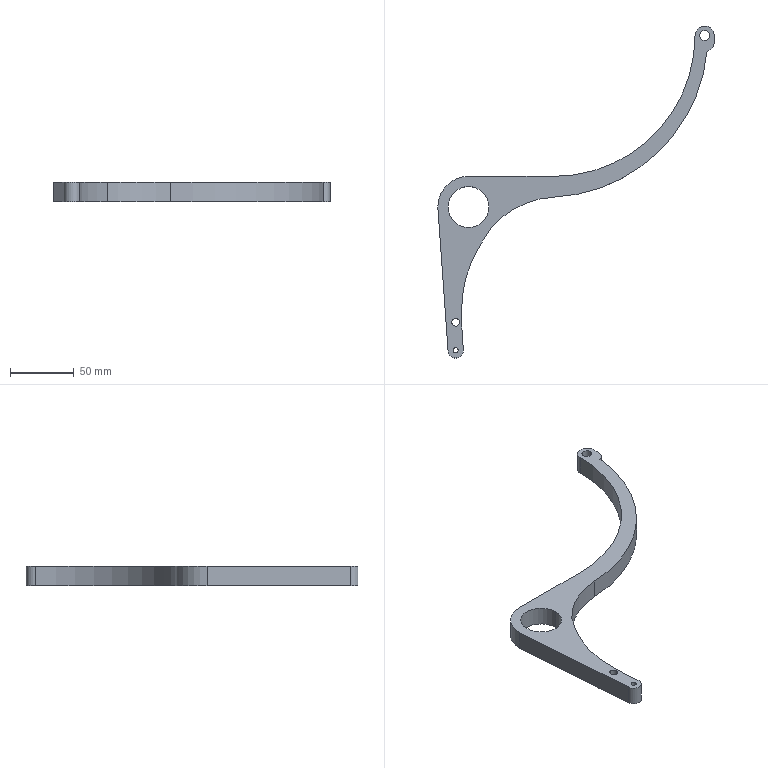Part | SolidWorks | features Extrusion 1 | 1 solid | 21 faces | box 216 x 259.5 x 15 mm | volume 91694 mm3 | cylinder 15 | plane 5 | spline 1 | commonest cylinder face diameters 4 x2 6 x2 7.838 x2 32 x2 12 x1 15 x1
STEP:
#1=CARTESIAN_POINT('',(-3.,22.,15.));
#2=VERTEX_POINT('',#1);
#3=CARTESIAN_POINT('',(3.,22.,15.));
#4=VERTEX_POINT('',#3);
#5=CARTESIAN_POINT('',(0.,22.,15.));
#6=DIRECTION('',(0.,0.,1.));
#7=DIRECTION('',(1.,0.,0.));
#8=AXIS2_PLACEMENT_3D('',#5,#6,#7);
#9=CIRCLE('',#8,3.);
#10=EDGE_CURVE('',#2,#4,#9,.T.);
#11=ORIENTED_EDGE('',*,*,#10,.T.);
#12=CARTESIAN_POINT('',(3.,22.,0.));
#13=VERTEX_POINT('',#12);
#14=CARTESIAN_POINT('',(3.,22.,15.));
#15=DIRECTION('',(0.,0.,-1.));
#16=VECTOR('',#15,1000.);
#17=LINE('',#14,#16);
#18=EDGE_CURVE('',#4,#13,#17,.T.);
#19=ORIENTED_EDGE('',*,*,#18,.T.);
#20=CARTESIAN_POINT('',(-3.,22.,0.));
#21=VERTEX_POINT('',#20);
#22=CARTESIAN_POINT('',(0.,22.,0.));
#23=DIRECTION('',(0.,0.,1.));
#24=DIRECTION('',(1.,0.,0.));
#25=AXIS2_PLACEMENT_3D('',#22,#23,#24);
#26=CIRCLE('',#25,3.);
#27=EDGE_CURVE('',#21,#13,#26,.T.);
#28=ORIENTED_EDGE('',*,*,#27,.F.);
#29=CARTESIAN_POINT('',(-3.,22.,15.));
#30=DIRECTION('',(0.,0.,-1.));
#31=VECTOR('',#30,1000.);
#32=LINE('',#29,#31);
#33=EDGE_CURVE('',#2,#21,#32,.T.);
#34=ORIENTED_EDGE('',*,*,#33,.F.);
#35=EDGE_LOOP('',(#11,#19,#28,#34));
#36=FACE_OUTER_BOUND('',#35,.T.);
#37=CARTESIAN_POINT('',(0.,22.,15.));
#38=DIRECTION('',(0.,0.,-1.));
#39=DIRECTION('',(-1.,0.,0.));
#40=AXIS2_PLACEMENT_3D('',#37,#38,#39);
#41=CYLINDRICAL_SURFACE('',#40,3.);
#42=ADVANCED_FACE('',(#36),#41,.F.);
#43=CARTESIAN_POINT('',(190.581,246.,15.));
#44=VERTEX_POINT('',#43);
#45=CARTESIAN_POINT('',(198.419,246.,15.));
#46=VERTEX_POINT('',#45);
#47=CARTESIAN_POINT('',(194.5,246.,15.));
#48=DIRECTION('',(0.,0.,1.));
#49=DIRECTION('',(1.,0.,0.));
#50=AXIS2_PLACEMENT_3D('',#47,#48,#49);
#51=CIRCLE('',#50,3.919);
#52=EDGE_CURVE('',#44,#46,#51,.T.);
#53=ORIENTED_EDGE('',*,*,#52,.T.);
#54=CARTESIAN_POINT('',(198.419,246.,0.));
#55=VERTEX_POINT('',#54);
#56=CARTESIAN_POINT('',(198.419,246.,15.));
#57=DIRECTION('',(0.,0.,-1.));
#58=VECTOR('',#57,1000.);
#59=LINE('',#56,#58);
#60=EDGE_CURVE('',#46,#55,#59,.T.);
#61=ORIENTED_EDGE('',*,*,#60,.T.);
#62=CARTESIAN_POINT('',(190.581,246.,0.));
#63=VERTEX_POINT('',#62);
#64=CARTESIAN_POINT('',(194.5,246.,0.));
#65=DIRECTION('',(0.,0.,1.));
#66=DIRECTION('',(1.,0.,0.));
#67=AXIS2_PLACEMENT_3D('',#64,#65,#66);
#68=CIRCLE('',#67,3.919);
#69=EDGE_CURVE('',#63,#55,#68,.T.);
#70=ORIENTED_EDGE('',*,*,#69,.F.);
#71=CARTESIAN_POINT('',(190.581,246.,15.));
#72=DIRECTION('',(0.,0.,-1.));
#73=VECTOR('',#72,1000.);
#74=LINE('',#71,#73);
#75=EDGE_CURVE('',#44,#63,#74,.T.);
#76=ORIENTED_EDGE('',*,*,#75,.F.);
#77=EDGE_LOOP('',(#53,#61,#70,#76));
#78=FACE_OUTER_BOUND('',#77,.T.);
#79=CARTESIAN_POINT('',(194.5,246.,15.));
#80=DIRECTION('',(0.,0.,-1.));
#81=DIRECTION('',(-1.,0.,0.));
#82=AXIS2_PLACEMENT_3D('',#79,#80,#81);
#83=CYLINDRICAL_SURFACE('',#82,3.919);
#84=ADVANCED_FACE('',(#78),#83,.F.);
#85=CARTESIAN_POINT('',(-6.,112.,15.));
#86=VERTEX_POINT('',#85);
#87=CARTESIAN_POINT('',(26.,112.,15.));
#88=VERTEX_POINT('',#87);
#89=CARTESIAN_POINT('',(10.,112.,15.));
#90=DIRECTION('',(0.,0.,1.));
#91=DIRECTION('',(1.,0.,0.));
#92=AXIS2_PLACEMENT_3D('',#89,#90,#91);
#93=CIRCLE('',#92,16.);
#94=EDGE_CURVE('',#86,#88,#93,.T.);
#95=ORIENTED_EDGE('',*,*,#94,.T.);
#96=CARTESIAN_POINT('',(26.,112.,0.));
#97=VERTEX_POINT('',#96);
#98=CARTESIAN_POINT('',(26.,112.,15.));
#99=DIRECTION('',(0.,0.,-1.));
#100=VECTOR('',#99,1000.);
#101=LINE('',#98,#100);
#102=EDGE_CURVE('',#88,#97,#101,.T.);
#103=ORIENTED_EDGE('',*,*,#102,.T.);
#104=CARTESIAN_POINT('',(-6.,112.,0.));
#105=VERTEX_POINT('',#104);
#106=CARTESIAN_POINT('',(10.,112.,0.));
#107=DIRECTION('',(0.,0.,1.));
#108=DIRECTION('',(1.,0.,0.));
#109=AXIS2_PLACEMENT_3D('',#106,#107,#108);
#110=CIRCLE('',#109,16.);
#111=EDGE_CURVE('',#105,#97,#110,.T.);
#112=ORIENTED_EDGE('',*,*,#111,.F.);
#113=CARTESIAN_POINT('',(-6.,112.,15.));
#114=DIRECTION('',(0.,0.,-1.));
#115=VECTOR('',#114,1000.);
#116=LINE('',#113,#115);
#117=EDGE_CURVE('',#86,#105,#116,.T.);
#118=ORIENTED_EDGE('',*,*,#117,.F.);
#119=EDGE_LOOP('',(#95,#103,#112,#118));
#120=FACE_OUTER_BOUND('',#119,.T.);
#121=CARTESIAN_POINT('',(10.,112.,15.));
#122=DIRECTION('',(0.,0.,-1.));
#123=DIRECTION('',(-1.,0.,0.));
#124=AXIS2_PLACEMENT_3D('',#121,#122,#123);
#125=CYLINDRICAL_SURFACE('',#124,16.);
#126=ADVANCED_FACE('',(#120),#125,.F.);
#127=CARTESIAN_POINT('',(-2.,0.,15.));
#128=VERTEX_POINT('',#127);
#129=CARTESIAN_POINT('',(2.,0.,15.));
#130=VERTEX_POINT('',#129);
#131=CARTESIAN_POINT('',(0.,0.,15.));
#132=DIRECTION('',(0.,0.,1.));
#133=DIRECTION('',(1.,0.,0.));
#134=AXIS2_PLACEMENT_3D('',#131,#132,#133);
#135=CIRCLE('',#134,2.);
#136=EDGE_CURVE('',#128,#130,#135,.T.);
#137=ORIENTED_EDGE('',*,*,#136,.T.);
#138=CARTESIAN_POINT('',(2.,0.,0.));
#139=VERTEX_POINT('',#138);
#140=CARTESIAN_POINT('',(2.,0.,15.));
#141=DIRECTION('',(0.,0.,-1.));
#142=VECTOR('',#141,1000.);
#143=LINE('',#140,#142);
#144=EDGE_CURVE('',#130,#139,#143,.T.);
#145=ORIENTED_EDGE('',*,*,#144,.T.);
#146=CARTESIAN_POINT('',(-2.,0.,0.));
#147=VERTEX_POINT('',#146);
#148=CARTESIAN_POINT('',(0.,0.,0.));
#149=DIRECTION('',(0.,0.,1.));
#150=DIRECTION('',(1.,0.,0.));
#151=AXIS2_PLACEMENT_3D('',#148,#149,#150);
#152=CIRCLE('',#151,2.);
#153=EDGE_CURVE('',#147,#139,#152,.T.);
#154=ORIENTED_EDGE('',*,*,#153,.F.);
#155=CARTESIAN_POINT('',(-2.,0.,15.));
#156=DIRECTION('',(0.,0.,-1.));
#157=VECTOR('',#156,1000.);
#158=LINE('',#155,#157);
#159=EDGE_CURVE('',#128,#147,#158,.T.);
#160=ORIENTED_EDGE('',*,*,#159,.F.);
#161=EDGE_LOOP('',(#137,#145,#154,#160));
#162=FACE_OUTER_BOUND('',#161,.T.);
#163=CARTESIAN_POINT('',(0.,0.,15.));
#164=DIRECTION('',(0.,0.,-1.));
#165=DIRECTION('',(-1.,0.,0.));
#166=AXIS2_PLACEMENT_3D('',#163,#164,#165);
#167=CYLINDRICAL_SURFACE('',#166,2.);
#168=ADVANCED_FACE('',(#162),#167,.F.);
#169=ORIENTED_EDGE('',*,*,#52,.F.);
#170=CARTESIAN_POINT('',(194.5,246.,15.));
#171=DIRECTION('',(0.,0.,1.));
#172=DIRECTION('',(1.,0.,0.));
#173=AXIS2_PLACEMENT_3D('',#170,#171,#172);
#174=CIRCLE('',#173,3.919);
#175=EDGE_CURVE('',#46,#44,#174,.T.);
#176=ORIENTED_EDGE('',*,*,#175,.F.);
#177=EDGE_LOOP('',(#169,#176));
#178=FACE_BOUND('',#177,.T.);
#179=ORIENTED_EDGE('',*,*,#136,.F.);
#180=CARTESIAN_POINT('',(0.,0.,15.));
#181=DIRECTION('',(0.,0.,1.));
#182=DIRECTION('',(1.,0.,0.));
#183=AXIS2_PLACEMENT_3D('',#180,#181,#182);
#184=CIRCLE('',#183,2.);
#185=EDGE_CURVE('',#130,#128,#184,.T.);
#186=ORIENTED_EDGE('',*,*,#185,.F.);
#187=EDGE_LOOP('',(#179,#186));
#188=FACE_BOUND('',#187,.T.);
#189=CARTESIAN_POINT('',(10.,136.,15.));
#190=VERTEX_POINT('',#189);
#191=CARTESIAN_POINT('',(-14.,112.,15.));
#192=VERTEX_POINT('',#191);
#193=CARTESIAN_POINT('',(10.,112.,15.));
#194=DIRECTION('',(0.,0.,1.));
#195=DIRECTION('',(1.,0.,0.));
#196=AXIS2_PLACEMENT_3D('',#193,#194,#195);
#197=CIRCLE('',#196,24.);
#198=EDGE_CURVE('',#190,#192,#197,.T.);
#199=ORIENTED_EDGE('',*,*,#198,.T.);
#200=CARTESIAN_POINT('',(-6.,0.,15.));
#201=VERTEX_POINT('',#200);
#202=CARTESIAN_POINT('',(-14.,112.,15.));
#203=DIRECTION('',(0.07125,-0.9975,0.));
#204=VECTOR('',#203,1000.);
#205=LINE('',#202,#204);
#206=EDGE_CURVE('',#192,#201,#205,.T.);
#207=ORIENTED_EDGE('',*,*,#206,.T.);
#208=CARTESIAN_POINT('',(6.,0.,15.));
#209=VERTEX_POINT('',#208);
#210=CARTESIAN_POINT('',(0.,0.,15.));
#211=DIRECTION('',(0.,0.,1.));
#212=DIRECTION('',(1.,0.,0.));
#213=AXIS2_PLACEMENT_3D('',#210,#211,#212);
#214=CIRCLE('',#213,6.);
#215=EDGE_CURVE('',#201,#209,#214,.T.);
#216=ORIENTED_EDGE('',*,*,#215,.T.);
#217=CARTESIAN_POINT('',(28.005,96.131,15.));
#218=VERTEX_POINT('',#217);
#219=CARTESIAN_POINT('',(6.,0.,15.));
#220=CARTESIAN_POINT('',(1.589,45.681,15.));
#221=CARTESIAN_POINT('',(5.604,63.643,15.));
#222=CARTESIAN_POINT('',(28.005,96.131,15.));
#223=B_SPLINE_CURVE_WITH_KNOTS('',3,(#219,#220,#221,#222),.UNSPECIFIED.,.F.,.F.,(4,4),(0.,0.7882),.UNSPECIFIED.);
#224=EDGE_CURVE('',#209,#218,#223,.T.);
#225=ORIENTED_EDGE('',*,*,#224,.T.);
#226=CARTESIAN_POINT('',(77.,119.767,15.));
#227=VERTEX_POINT('',#226);
#228=CARTESIAN_POINT('',(80.543,49.825,15.));
#229=DIRECTION('',(0.,0.,-1.));
#230=DIRECTION('',(1.,0.,0.));
#231=AXIS2_PLACEMENT_3D('',#228,#229,#230);
#232=CIRCLE('',#231,70.032);
#233=EDGE_CURVE('',#218,#227,#232,.T.);
#234=ORIENTED_EDGE('',*,*,#233,.T.);
#235=CARTESIAN_POINT('',(196.38,233.495,15.));
#236=VERTEX_POINT('',#235);
#237=CARTESIAN_POINT('',(70.606,246.,15.));
#238=DIRECTION('',(0.,0.,1.));
#239=DIRECTION('',(1.,0.,0.));
#240=AXIS2_PLACEMENT_3D('',#237,#238,#239);
#241=CIRCLE('',#240,126.394);
#242=EDGE_CURVE('',#227,#236,#241,.T.);
#243=ORIENTED_EDGE('',*,*,#242,.T.);
#244=CARTESIAN_POINT('',(202.,241.,15.));
#245=VERTEX_POINT('',#244);
#246=CARTESIAN_POINT('',(194.179,241.,15.));
#247=DIRECTION('',(0.,0.,1.));
#248=DIRECTION('',(1.,0.,0.));
#249=AXIS2_PLACEMENT_3D('',#246,#247,#248);
#250=CIRCLE('',#249,7.821);
#251=EDGE_CURVE('',#236,#245,#250,.T.);
#252=ORIENTED_EDGE('',*,*,#251,.T.);
#253=CARTESIAN_POINT('',(202.,246.,15.));
#254=VERTEX_POINT('',#253);
#255=CARTESIAN_POINT('',(202.,246.,15.));
#256=DIRECTION('',(0.,1.,0.));
#257=VECTOR('',#256,1000.);
#258=LINE('',#255,#257);
#259=EDGE_CURVE('',#245,#254,#258,.T.);
#260=ORIENTED_EDGE('',*,*,#259,.T.);
#261=CARTESIAN_POINT('',(187.,246.,15.));
#262=VERTEX_POINT('',#261);
#263=CARTESIAN_POINT('',(194.5,246.,15.));
#264=DIRECTION('',(0.,0.,1.));
#265=DIRECTION('',(1.,0.,0.));
#266=AXIS2_PLACEMENT_3D('',#263,#264,#265);
#267=CIRCLE('',#266,7.5);
#268=EDGE_CURVE('',#254,#262,#267,.T.);
#269=ORIENTED_EDGE('',*,*,#268,.T.);
#270=CARTESIAN_POINT('',(77.,136.,15.));
#271=VERTEX_POINT('',#270);
#272=CARTESIAN_POINT('',(77.,246.,15.));
#273=DIRECTION('',(0.,0.,-1.));
#274=DIRECTION('',(1.,0.,0.));
#275=AXIS2_PLACEMENT_3D('',#272,#273,#274);
#276=CIRCLE('',#275,110.);
#277=EDGE_CURVE('',#262,#271,#276,.T.);
#278=ORIENTED_EDGE('',*,*,#277,.T.);
#279=CARTESIAN_POINT('',(10.,136.,15.));
#280=DIRECTION('',(-1.,0.,0.));
#281=VECTOR('',#280,1000.);
#282=LINE('',#279,#281);
#283=EDGE_CURVE('',#271,#190,#282,.T.);
#284=ORIENTED_EDGE('',*,*,#283,.T.);
#285=EDGE_LOOP('',(#199,#207,#216,#225,#234,#243,#252,#260,#269,#278,#284));
#286=FACE_OUTER_BOUND('',#285,.T.);
#287=ORIENTED_EDGE('',*,*,#94,.F.);
#288=CARTESIAN_POINT('',(10.,112.,15.));
#289=DIRECTION('',(0.,0.,1.));
#290=DIRECTION('',(1.,0.,0.));
#291=AXIS2_PLACEMENT_3D('',#288,#289,#290);
#292=CIRCLE('',#291,16.);
#293=EDGE_CURVE('',#88,#86,#292,.T.);
#294=ORIENTED_EDGE('',*,*,#293,.F.);
#295=EDGE_LOOP('',(#287,#294));
#296=FACE_BOUND('',#295,.T.);
#297=ORIENTED_EDGE('',*,*,#10,.F.);
#298=CARTESIAN_POINT('',(0.,22.,15.));
#299=DIRECTION('',(0.,0.,1.));
#300=DIRECTION('',(1.,0.,0.));
#301=AXIS2_PLACEMENT_3D('',#298,#299,#300);
#302=CIRCLE('',#301,3.);
#303=EDGE_CURVE('',#4,#2,#302,.T.);
#304=ORIENTED_EDGE('',*,*,#303,.F.);
#305=EDGE_LOOP('',(#297,#304));
#306=FACE_BOUND('',#305,.T.);
#307=CARTESIAN_POINT('',(10.,112.,15.));
#308=DIRECTION('',(0.,0.,1.));
#309=DIRECTION('',(1.,0.,0.));
#310=AXIS2_PLACEMENT_3D('',#307,#308,#309);
#311=PLANE('',#310);
#312=ADVANCED_FACE('',(#178,#188,#286,#296,#306),#311,.T.);
#313=CARTESIAN_POINT('',(10.,136.,0.));
#314=VERTEX_POINT('',#313);
#315=CARTESIAN_POINT('',(-14.,112.,0.));
#316=VERTEX_POINT('',#315);
#317=CARTESIAN_POINT('',(10.,112.,0.));
#318=DIRECTION('',(0.,0.,1.));
#319=DIRECTION('',(1.,0.,0.));
#320=AXIS2_PLACEMENT_3D('',#317,#318,#319);
#321=CIRCLE('',#320,24.);
#322=EDGE_CURVE('',#314,#316,#321,.T.);
#323=ORIENTED_EDGE('',*,*,#322,.F.);
#324=CARTESIAN_POINT('',(77.,136.,0.));
#325=VERTEX_POINT('',#324);
#326=CARTESIAN_POINT('',(10.,136.,0.));
#327=DIRECTION('',(-1.,0.,0.));
#328=VECTOR('',#327,1000.);
#329=LINE('',#326,#328);
#330=EDGE_CURVE('',#325,#314,#329,.T.);
#331=ORIENTED_EDGE('',*,*,#330,.F.);
#332=CARTESIAN_POINT('',(187.,246.,0.));
#333=VERTEX_POINT('',#332);
#334=CARTESIAN_POINT('',(77.,246.,0.));
#335=DIRECTION('',(0.,0.,-1.));
#336=DIRECTION('',(1.,0.,0.));
#337=AXIS2_PLACEMENT_3D('',#334,#335,#336);
#338=CIRCLE('',#337,110.);
#339=EDGE_CURVE('',#333,#325,#338,.T.);
#340=ORIENTED_EDGE('',*,*,#339,.F.);
#341=CARTESIAN_POINT('',(202.,246.,0.));
#342=VERTEX_POINT('',#341);
#343=CARTESIAN_POINT('',(194.5,246.,0.));
#344=DIRECTION('',(0.,0.,1.));
#345=DIRECTION('',(1.,0.,0.));
#346=AXIS2_PLACEMENT_3D('',#343,#344,#345);
#347=CIRCLE('',#346,7.5);
#348=EDGE_CURVE('',#342,#333,#347,.T.);
#349=ORIENTED_EDGE('',*,*,#348,.F.);
#350=CARTESIAN_POINT('',(202.,241.,0.));
#351=VERTEX_POINT('',#350);
#352=CARTESIAN_POINT('',(202.,246.,0.));
#353=DIRECTION('',(0.,1.,0.));
#354=VECTOR('',#353,1000.);
#355=LINE('',#352,#354);
#356=EDGE_CURVE('',#351,#342,#355,.T.);
#357=ORIENTED_EDGE('',*,*,#356,.F.);
#358=CARTESIAN_POINT('',(196.38,233.495,0.));
#359=VERTEX_POINT('',#358);
#360=CARTESIAN_POINT('',(194.179,241.,0.));
#361=DIRECTION('',(0.,0.,1.));
#362=DIRECTION('',(1.,0.,0.));
#363=AXIS2_PLACEMENT_3D('',#360,#361,#362);
#364=CIRCLE('',#363,7.821);
#365=EDGE_CURVE('',#359,#351,#364,.T.);
#366=ORIENTED_EDGE('',*,*,#365,.F.);
#367=CARTESIAN_POINT('',(77.,119.767,0.));
#368=VERTEX_POINT('',#367);
#369=CARTESIAN_POINT('',(70.606,246.,0.));
#370=DIRECTION('',(0.,0.,1.));
#371=DIRECTION('',(1.,0.,0.));
#372=AXIS2_PLACEMENT_3D('',#369,#370,#371);
#373=CIRCLE('',#372,126.394);
#374=EDGE_CURVE('',#368,#359,#373,.T.);
#375=ORIENTED_EDGE('',*,*,#374,.F.);
#376=CARTESIAN_POINT('',(28.005,96.131,0.));
#377=VERTEX_POINT('',#376);
#378=CARTESIAN_POINT('',(80.543,49.825,0.));
#379=DIRECTION('',(0.,0.,-1.));
#380=DIRECTION('',(1.,0.,0.));
#381=AXIS2_PLACEMENT_3D('',#378,#379,#380);
#382=CIRCLE('',#381,70.032);
#383=EDGE_CURVE('',#377,#368,#382,.T.);
#384=ORIENTED_EDGE('',*,*,#383,.F.);
#385=CARTESIAN_POINT('',(6.,0.,0.));
#386=VERTEX_POINT('',#385);
#387=CARTESIAN_POINT('',(6.,0.,0.));
#388=CARTESIAN_POINT('',(1.589,45.681,0.));
#389=CARTESIAN_POINT('',(5.604,63.643,0.));
#390=CARTESIAN_POINT('',(28.005,96.131,0.));
#391=B_SPLINE_CURVE_WITH_KNOTS('',3,(#387,#388,#389,#390),.UNSPECIFIED.,.F.,.F.,(4,4),(0.,0.7882),.UNSPECIFIED.);
#392=EDGE_CURVE('',#386,#377,#391,.T.);
#393=ORIENTED_EDGE('',*,*,#392,.F.);
#394=CARTESIAN_POINT('',(-6.,0.,0.));
#395=VERTEX_POINT('',#394);
#396=CARTESIAN_POINT('',(0.,0.,0.));
#397=DIRECTION('',(0.,0.,1.));
#398=DIRECTION('',(1.,0.,0.));
#399=AXIS2_PLACEMENT_3D('',#396,#397,#398);
#400=CIRCLE('',#399,6.);
#401=EDGE_CURVE('',#395,#386,#400,.T.);
#402=ORIENTED_EDGE('',*,*,#401,.F.);
#403=CARTESIAN_POINT('',(-14.,112.,0.));
#404=DIRECTION('',(0.07125,-0.9975,0.));
#405=VECTOR('',#404,1000.);
#406=LINE('',#403,#405);
#407=EDGE_CURVE('',#316,#395,#406,.T.);
#408=ORIENTED_EDGE('',*,*,#407,.F.);
#409=EDGE_LOOP('',(#323,#331,#340,#349,#357,#366,#375,#384,#393,#402,#408));
#410=FACE_OUTER_BOUND('',#409,.T.);
#411=ORIENTED_EDGE('',*,*,#153,.T.);
#412=CARTESIAN_POINT('',(0.,0.,0.));
#413=DIRECTION('',(0.,0.,1.));
#414=DIRECTION('',(1.,0.,0.));
#415=AXIS2_PLACEMENT_3D('',#412,#413,#414);
#416=CIRCLE('',#415,2.);
#417=EDGE_CURVE('',#139,#147,#416,.T.);
#418=ORIENTED_EDGE('',*,*,#417,.T.);
#419=EDGE_LOOP('',(#411,#418));
#420=FACE_BOUND('',#419,.T.);
#421=ORIENTED_EDGE('',*,*,#111,.T.);
#422=CARTESIAN_POINT('',(10.,112.,0.));
#423=DIRECTION('',(0.,0.,1.));
#424=DIRECTION('',(1.,0.,0.));
#425=AXIS2_PLACEMENT_3D('',#422,#423,#424);
#426=CIRCLE('',#425,16.);
#427=EDGE_CURVE('',#97,#105,#426,.T.);
#428=ORIENTED_EDGE('',*,*,#427,.T.);
#429=EDGE_LOOP('',(#421,#428));
#430=FACE_BOUND('',#429,.T.);
#431=ORIENTED_EDGE('',*,*,#69,.T.);
#432=CARTESIAN_POINT('',(194.5,246.,0.));
#433=DIRECTION('',(0.,0.,1.));
#434=DIRECTION('',(1.,0.,0.));
#435=AXIS2_PLACEMENT_3D('',#432,#433,#434);
#436=CIRCLE('',#435,3.919);
#437=EDGE_CURVE('',#55,#63,#436,.T.);
#438=ORIENTED_EDGE('',*,*,#437,.T.);
#439=EDGE_LOOP('',(#431,#438));
#440=FACE_BOUND('',#439,.T.);
#441=ORIENTED_EDGE('',*,*,#27,.T.);
#442=CARTESIAN_POINT('',(0.,22.,0.));
#443=DIRECTION('',(0.,0.,1.));
#444=DIRECTION('',(1.,0.,0.));
#445=AXIS2_PLACEMENT_3D('',#442,#443,#444);
#446=CIRCLE('',#445,3.);
#447=EDGE_CURVE('',#13,#21,#446,.T.);
#448=ORIENTED_EDGE('',*,*,#447,.T.);
#449=EDGE_LOOP('',(#441,#448));
#450=FACE_BOUND('',#449,.T.);
#451=CARTESIAN_POINT('',(10.,112.,0.));
#452=DIRECTION('',(0.,0.,1.));
#453=DIRECTION('',(1.,0.,0.));
#454=AXIS2_PLACEMENT_3D('',#451,#452,#453);
#455=PLANE('',#454);
#456=ADVANCED_FACE('',(#410,#420,#430,#440,#450),#455,.F.);
#457=ORIENTED_EDGE('',*,*,#322,.T.);
#458=CARTESIAN_POINT('',(-14.,112.,15.));
#459=DIRECTION('',(0.,0.,-1.));
#460=VECTOR('',#459,1000.);
#461=LINE('',#458,#460);
#462=EDGE_CURVE('',#192,#316,#461,.T.);
#463=ORIENTED_EDGE('',*,*,#462,.F.);
#464=ORIENTED_EDGE('',*,*,#198,.F.);
#465=CARTESIAN_POINT('',(10.,136.,15.));
#466=DIRECTION('',(0.,0.,-1.));
#467=VECTOR('',#466,1000.);
#468=LINE('',#465,#467);
#469=EDGE_CURVE('',#190,#314,#468,.T.);
#470=ORIENTED_EDGE('',*,*,#469,.T.);
#471=EDGE_LOOP('',(#457,#463,#464,#470));
#472=FACE_OUTER_BOUND('',#471,.T.);
#473=CARTESIAN_POINT('',(10.,112.,15.));
#474=DIRECTION('',(0.,0.,-1.));
#475=DIRECTION('',(-1.,0.,0.));
#476=AXIS2_PLACEMENT_3D('',#473,#474,#475);
#477=CYLINDRICAL_SURFACE('',#476,24.);
#478=ADVANCED_FACE('',(#472),#477,.T.);
#479=ORIENTED_EDGE('',*,*,#407,.T.);
#480=CARTESIAN_POINT('',(-6.,0.,15.));
#481=DIRECTION('',(0.,0.,-1.));
#482=VECTOR('',#481,1000.);
#483=LINE('',#480,#482);
#484=EDGE_CURVE('',#201,#395,#483,.T.);
#485=ORIENTED_EDGE('',*,*,#484,.F.);
#486=ORIENTED_EDGE('',*,*,#206,.F.);
#487=ORIENTED_EDGE('',*,*,#462,.T.);
#488=EDGE_LOOP('',(#479,#485,#486,#487));
#489=FACE_OUTER_BOUND('',#488,.T.);
#490=CARTESIAN_POINT('',(-14.,112.,15.));
#491=DIRECTION('',(0.9975,0.07125,0.));
#492=DIRECTION('',(-0.07125,0.9975,0.));
#493=AXIS2_PLACEMENT_3D('',#490,#491,#492);
#494=PLANE('',#493);
#495=ADVANCED_FACE('',(#489),#494,.F.);
#496=ORIENTED_EDGE('',*,*,#401,.T.);
#497=CARTESIAN_POINT('',(6.,0.,15.));
#498=DIRECTION('',(0.,0.,-1.));
#499=VECTOR('',#498,1000.);
#500=LINE('',#497,#499);
#501=EDGE_CURVE('',#209,#386,#500,.T.);
#502=ORIENTED_EDGE('',*,*,#501,.F.);
#503=ORIENTED_EDGE('',*,*,#215,.F.);
#504=ORIENTED_EDGE('',*,*,#484,.T.);
#505=EDGE_LOOP('',(#496,#502,#503,#504));
#506=FACE_OUTER_BOUND('',#505,.T.);
#507=CARTESIAN_POINT('',(0.,0.,15.));
#508=DIRECTION('',(0.,0.,-1.));
#509=DIRECTION('',(-1.,0.,0.));
#510=AXIS2_PLACEMENT_3D('',#507,#508,#509);
#511=CYLINDRICAL_SURFACE('',#510,6.);
#512=ADVANCED_FACE('',(#506),#511,.T.);
#513=ORIENTED_EDGE('',*,*,#392,.T.);
#514=CARTESIAN_POINT('',(28.005,96.131,15.));
#515=DIRECTION('',(0.,0.,-1.));
#516=VECTOR('',#515,1000.);
#517=LINE('',#514,#516);
#518=EDGE_CURVE('',#218,#377,#517,.T.);
#519=ORIENTED_EDGE('',*,*,#518,.F.);
#520=ORIENTED_EDGE('',*,*,#224,.F.);
#521=ORIENTED_EDGE('',*,*,#501,.T.);
#522=EDGE_LOOP('',(#513,#519,#520,#521));
#523=FACE_OUTER_BOUND('',#522,.T.);
#524=CARTESIAN_POINT('',(6.,0.,15.));
#525=CARTESIAN_POINT('',(6.,0.,0.));
#526=CARTESIAN_POINT('',(1.589,45.681,15.));
#527=CARTESIAN_POINT('',(1.589,45.681,0.));
#528=CARTESIAN_POINT('',(5.604,63.643,15.));
#529=CARTESIAN_POINT('',(5.604,63.643,0.));
#530=CARTESIAN_POINT('',(28.005,96.131,15.));
#531=CARTESIAN_POINT('',(28.005,96.131,0.));
#532=B_SPLINE_SURFACE_WITH_KNOTS('',3,1,((#524,#525),(#526,#527),(#528,#529),(#530,#531)),.UNSPECIFIED.,.F.,.F.,.F.,(4,4),(2,2),(0.,0.7882),(0.,1.),.UNSPECIFIED.);
#533=ADVANCED_FACE('',(#523),#532,.F.);
#534=ORIENTED_EDGE('',*,*,#383,.T.);
#535=CARTESIAN_POINT('',(77.,119.767,15.));
#536=DIRECTION('',(0.,0.,-1.));
#537=VECTOR('',#536,1000.);
#538=LINE('',#535,#537);
#539=EDGE_CURVE('',#227,#368,#538,.T.);
#540=ORIENTED_EDGE('',*,*,#539,.F.);
#541=ORIENTED_EDGE('',*,*,#233,.F.);
#542=ORIENTED_EDGE('',*,*,#518,.T.);
#543=EDGE_LOOP('',(#534,#540,#541,#542));
#544=FACE_OUTER_BOUND('',#543,.T.);
#545=CARTESIAN_POINT('',(80.543,49.825,15.));
#546=DIRECTION('',(0.,0.,-1.));
#547=DIRECTION('',(-1.,0.,0.));
#548=AXIS2_PLACEMENT_3D('',#545,#546,#547);
#549=CYLINDRICAL_SURFACE('',#548,70.032);
#550=ADVANCED_FACE('',(#544),#549,.F.);
#551=ORIENTED_EDGE('',*,*,#374,.T.);
#552=CARTESIAN_POINT('',(196.38,233.495,15.));
#553=DIRECTION('',(0.,0.,-1.));
#554=VECTOR('',#553,1000.);
#555=LINE('',#552,#554);
#556=EDGE_CURVE('',#236,#359,#555,.T.);
#557=ORIENTED_EDGE('',*,*,#556,.F.);
#558=ORIENTED_EDGE('',*,*,#242,.F.);
#559=ORIENTED_EDGE('',*,*,#539,.T.);
#560=EDGE_LOOP('',(#551,#557,#558,#559));
#561=FACE_OUTER_BOUND('',#560,.T.);
#562=CARTESIAN_POINT('',(70.606,246.,15.));
#563=DIRECTION('',(0.,0.,-1.));
#564=DIRECTION('',(-1.,0.,0.));
#565=AXIS2_PLACEMENT_3D('',#562,#563,#564);
#566=CYLINDRICAL_SURFACE('',#565,126.394);
#567=ADVANCED_FACE('',(#561),#566,.T.);
#568=ORIENTED_EDGE('',*,*,#365,.T.);
#569=CARTESIAN_POINT('',(202.,241.,15.));
#570=DIRECTION('',(0.,0.,-1.));
#571=VECTOR('',#570,1000.);
#572=LINE('',#569,#571);
#573=EDGE_CURVE('',#245,#351,#572,.T.);
#574=ORIENTED_EDGE('',*,*,#573,.F.);
#575=ORIENTED_EDGE('',*,*,#251,.F.);
#576=ORIENTED_EDGE('',*,*,#556,.T.);
#577=EDGE_LOOP('',(#568,#574,#575,#576));
#578=FACE_OUTER_BOUND('',#577,.T.);
#579=CARTESIAN_POINT('',(194.179,241.,15.));
#580=DIRECTION('',(0.,0.,-1.));
#581=DIRECTION('',(-1.,0.,0.));
#582=AXIS2_PLACEMENT_3D('',#579,#580,#581);
#583=CYLINDRICAL_SURFACE('',#582,7.821);
#584=ADVANCED_FACE('',(#578),#583,.T.);
#585=ORIENTED_EDGE('',*,*,#356,.T.);
#586=CARTESIAN_POINT('',(202.,246.,15.));
#587=DIRECTION('',(0.,0.,-1.));
#588=VECTOR('',#587,1000.);
#589=LINE('',#586,#588);
#590=EDGE_CURVE('',#254,#342,#589,.T.);
#591=ORIENTED_EDGE('',*,*,#590,.F.);
#592=ORIENTED_EDGE('',*,*,#259,.F.);
#593=ORIENTED_EDGE('',*,*,#573,.T.);
#594=EDGE_LOOP('',(#585,#591,#592,#593));
#595=FACE_OUTER_BOUND('',#594,.T.);
#596=CARTESIAN_POINT('',(202.,246.,15.));
#597=DIRECTION('',(-1.,0.,0.));
#598=DIRECTION('',(0.,0.,1.));
#599=AXIS2_PLACEMENT_3D('',#596,#597,#598);
#600=PLANE('',#599);
#601=ADVANCED_FACE('',(#595),#600,.F.);
#602=ORIENTED_EDGE('',*,*,#348,.T.);
#603=CARTESIAN_POINT('',(187.,246.,15.));
#604=DIRECTION('',(0.,0.,-1.));
#605=VECTOR('',#604,1000.);
#606=LINE('',#603,#605);
#607=EDGE_CURVE('',#262,#333,#606,.T.);
#608=ORIENTED_EDGE('',*,*,#607,.F.);
#609=ORIENTED_EDGE('',*,*,#268,.F.);
#610=ORIENTED_EDGE('',*,*,#590,.T.);
#611=EDGE_LOOP('',(#602,#608,#609,#610));
#612=FACE_OUTER_BOUND('',#611,.T.);
#613=CARTESIAN_POINT('',(194.5,246.,15.));
#614=DIRECTION('',(0.,0.,-1.));
#615=DIRECTION('',(-1.,0.,0.));
#616=AXIS2_PLACEMENT_3D('',#613,#614,#615);
#617=CYLINDRICAL_SURFACE('',#616,7.5);
#618=ADVANCED_FACE('',(#612),#617,.T.);
#619=ORIENTED_EDGE('',*,*,#339,.T.);
#620=CARTESIAN_POINT('',(77.,136.,15.));
#621=DIRECTION('',(0.,0.,-1.));
#622=VECTOR('',#621,1000.);
#623=LINE('',#620,#622);
#624=EDGE_CURVE('',#271,#325,#623,.T.);
#625=ORIENTED_EDGE('',*,*,#624,.F.);
#626=ORIENTED_EDGE('',*,*,#277,.F.);
#627=ORIENTED_EDGE('',*,*,#607,.T.);
#628=EDGE_LOOP('',(#619,#625,#626,#627));
#629=FACE_OUTER_BOUND('',#628,.T.);
#630=CARTESIAN_POINT('',(77.,246.,15.));
#631=DIRECTION('',(0.,0.,-1.));
#632=DIRECTION('',(-1.,0.,0.));
#633=AXIS2_PLACEMENT_3D('',#630,#631,#632);
#634=CYLINDRICAL_SURFACE('',#633,110.);
#635=ADVANCED_FACE('',(#629),#634,.F.);
#636=ORIENTED_EDGE('',*,*,#330,.T.);
#637=ORIENTED_EDGE('',*,*,#469,.F.);
#638=ORIENTED_EDGE('',*,*,#283,.F.);
#639=ORIENTED_EDGE('',*,*,#624,.T.);
#640=EDGE_LOOP('',(#636,#637,#638,#639));
#641=FACE_OUTER_BOUND('',#640,.T.);
#642=CARTESIAN_POINT('',(10.,136.,15.));
#643=DIRECTION('',(0.,-1.,0.));
#644=DIRECTION('',(0.,0.,-1.));
#645=AXIS2_PLACEMENT_3D('',#642,#643,#644);
#646=PLANE('',#645);
#647=ADVANCED_FACE('',(#641),#646,.F.);
#648=ORIENTED_EDGE('',*,*,#144,.F.);
#649=ORIENTED_EDGE('',*,*,#185,.T.);
#650=ORIENTED_EDGE('',*,*,#159,.T.);
#651=ORIENTED_EDGE('',*,*,#417,.F.);
#652=EDGE_LOOP('',(#648,#649,#650,#651));
#653=FACE_OUTER_BOUND('',#652,.T.);
#654=CARTESIAN_POINT('',(0.,0.,15.));
#655=DIRECTION('',(0.,0.,-1.));
#656=DIRECTION('',(-1.,0.,0.));
#657=AXIS2_PLACEMENT_3D('',#654,#655,#656);
#658=CYLINDRICAL_SURFACE('',#657,2.);
#659=ADVANCED_FACE('',(#653),#658,.F.);
#660=ORIENTED_EDGE('',*,*,#102,.F.);
#661=ORIENTED_EDGE('',*,*,#293,.T.);
#662=ORIENTED_EDGE('',*,*,#117,.T.);
#663=ORIENTED_EDGE('',*,*,#427,.F.);
#664=EDGE_LOOP('',(#660,#661,#662,#663));
#665=FACE_OUTER_BOUND('',#664,.T.);
#666=CARTESIAN_POINT('',(10.,112.,15.));
#667=DIRECTION('',(0.,0.,-1.));
#668=DIRECTION('',(-1.,0.,0.));
#669=AXIS2_PLACEMENT_3D('',#666,#667,#668);
#670=CYLINDRICAL_SURFACE('',#669,16.);
#671=ADVANCED_FACE('',(#665),#670,.F.);
#672=ORIENTED_EDGE('',*,*,#60,.F.);
#673=ORIENTED_EDGE('',*,*,#175,.T.);
#674=ORIENTED_EDGE('',*,*,#75,.T.);
#675=ORIENTED_EDGE('',*,*,#437,.F.);
#676=EDGE_LOOP('',(#672,#673,#674,#675));
#677=FACE_OUTER_BOUND('',#676,.T.);
#678=CARTESIAN_POINT('',(194.5,246.,15.));
#679=DIRECTION('',(0.,0.,-1.));
#680=DIRECTION('',(-1.,0.,0.));
#681=AXIS2_PLACEMENT_3D('',#678,#679,#680);
#682=CYLINDRICAL_SURFACE('',#681,3.919);
#683=ADVANCED_FACE('',(#677),#682,.F.);
#684=ORIENTED_EDGE('',*,*,#18,.F.);
#685=ORIENTED_EDGE('',*,*,#303,.T.);
#686=ORIENTED_EDGE('',*,*,#33,.T.);
#687=ORIENTED_EDGE('',*,*,#447,.F.);
#688=EDGE_LOOP('',(#684,#685,#686,#687));
#689=FACE_OUTER_BOUND('',#688,.T.);
#690=CARTESIAN_POINT('',(0.,22.,15.));
#691=DIRECTION('',(0.,0.,-1.));
#692=DIRECTION('',(-1.,0.,0.));
#693=AXIS2_PLACEMENT_3D('',#690,#691,#692);
#694=CYLINDRICAL_SURFACE('',#693,3.);
#695=ADVANCED_FACE('',(#689),#694,.F.);
#696=CLOSED_SHELL('',(#42,#84,#126,#168,#312,#456,#478,#495,#512,#533,#550,#567,#584,#601,#618,#635,#647,#659,#671,#683,#695));
#697=MANIFOLD_SOLID_BREP('',#696);
#698=CARTESIAN_POINT('',(0.,0.,0.));
#699=DIRECTION('',(0.,0.,1.));
#700=DIRECTION('',(1.,0.,0.));
#701=AXIS2_PLACEMENT_3D('',#698,#699,#700);
#702=(LENGTH_UNIT()NAMED_UNIT(*)SI_UNIT(.MILLI.,.METRE.));
#703=UNCERTAINTY_MEASURE_WITH_UNIT(LENGTH_MEASURE(0.00001),#702,'','');
#704=(NAMED_UNIT(*)PLANE_ANGLE_UNIT()SI_UNIT($,.RADIAN.));
#705=(NAMED_UNIT(*)SI_UNIT($,.STERADIAN.)SOLID_ANGLE_UNIT());
#706=(GEOMETRIC_REPRESENTATION_CONTEXT(3)GLOBAL_UNCERTAINTY_ASSIGNED_CONTEXT((#703))GLOBAL_UNIT_ASSIGNED_CONTEXT((#702,#704,#705))REPRESENTATION_CONTEXT('',''));
#707=ADVANCED_BREP_SHAPE_REPRESENTATION('',(#697,#701),#706);